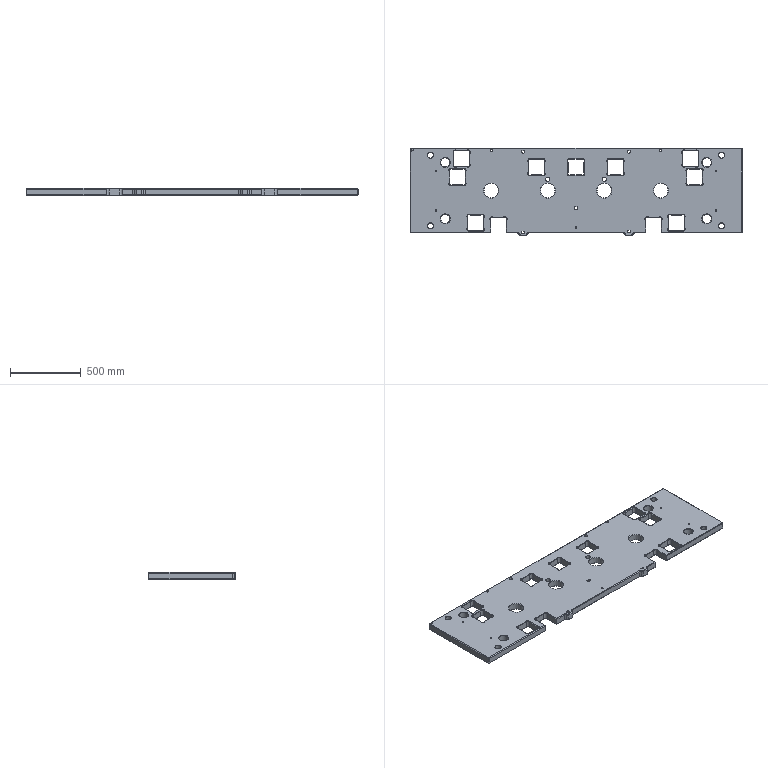Part | STEP file | solid 226 | 1 solid | 494 faces | box 2350 x 620 x 50 mm | volume 60712018 mm3 | plane 209 | cone 172 | cylinder 112 | other 1 | commonest cylinder face diameters 26 x48 14 x22 5 x6 10.2 x4 22 x4 40 x4